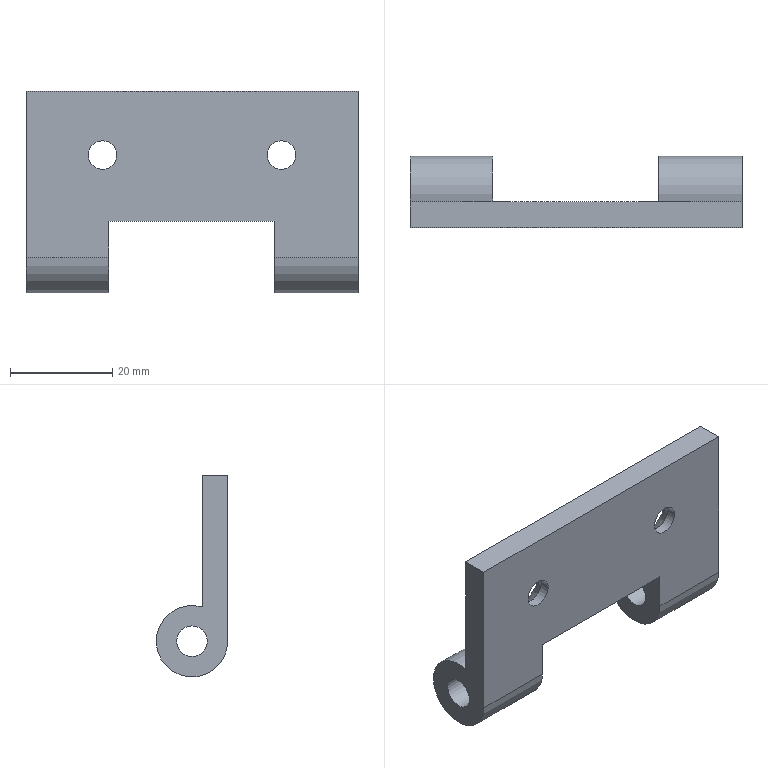Part | NX | 1 solid | 16 faces | box 65 x 14 x 39.5 mm | volume 12285 mm3 | plane 8 | cylinder 6 | cone 2 | commonest cylinder face diameters 5.6 x2 6 x2 14 x2
STEP:
#1=CARTESIAN_POINT('',(50.,0.,22.8));
#2=VERTEX_POINT('',#1);
#3=CARTESIAN_POINT('',(50.,0.,20.));
#4=DIRECTION('',(0.,1.,0.));
#5=DIRECTION('',(0.,0.,1.));
#6=AXIS2_PLACEMENT_3D('',#3,#4,#5);
#7=CIRCLE('',#6,2.8);
#8=EDGE_CURVE('',#2,#2,#7,.T.);
#9=ORIENTED_EDGE('',*,*,#8,.T.);
#10=EDGE_LOOP('',(#9));
#11=FACE_BOUND('',#10,.T.);
#12=CARTESIAN_POINT('',(16.25,0.,7.));
#13=VERTEX_POINT('',#12);
#14=CARTESIAN_POINT('',(48.75,0.,7.));
#15=VERTEX_POINT('',#14);
#16=CARTESIAN_POINT('',(65.,0.,7.));
#17=DIRECTION('',(1.,0.,0.));
#18=VECTOR('',#17,1000.);
#19=LINE('',#16,#18);
#20=EDGE_CURVE('',#13,#15,#19,.T.);
#21=ORIENTED_EDGE('',*,*,#20,.T.);
#22=CARTESIAN_POINT('',(48.75,0.,0.));
#23=VERTEX_POINT('',#22);
#24=CARTESIAN_POINT('',(48.75,0.,32.5));
#25=DIRECTION('',(0.,0.,-1.));
#26=VECTOR('',#25,1000.);
#27=LINE('',#24,#26);
#28=EDGE_CURVE('',#15,#23,#27,.T.);
#29=ORIENTED_EDGE('',*,*,#28,.T.);
#30=CARTESIAN_POINT('',(65.,0.,0.));
#31=VERTEX_POINT('',#30);
#32=CARTESIAN_POINT('',(65.,0.,0.));
#33=DIRECTION('',(-1.,0.,0.));
#34=VECTOR('',#33,1000.);
#35=LINE('',#32,#34);
#36=EDGE_CURVE('',#31,#23,#35,.T.);
#37=ORIENTED_EDGE('',*,*,#36,.F.);
#38=CARTESIAN_POINT('',(65.,0.,32.5));
#39=VERTEX_POINT('',#38);
#40=CARTESIAN_POINT('',(65.,0.,32.5));
#41=DIRECTION('',(0.,0.,-1.));
#42=VECTOR('',#41,1000.);
#43=LINE('',#40,#42);
#44=EDGE_CURVE('',#39,#31,#43,.T.);
#45=ORIENTED_EDGE('',*,*,#44,.F.);
#46=CARTESIAN_POINT('',(0.,0.,32.5));
#47=VERTEX_POINT('',#46);
#48=CARTESIAN_POINT('',(65.,0.,32.5));
#49=DIRECTION('',(-1.,0.,0.));
#50=VECTOR('',#49,1000.);
#51=LINE('',#48,#50);
#52=EDGE_CURVE('',#39,#47,#51,.T.);
#53=ORIENTED_EDGE('',*,*,#52,.T.);
#54=CARTESIAN_POINT('',(0.,0.,0.));
#55=VERTEX_POINT('',#54);
#56=CARTESIAN_POINT('',(0.,0.,32.5));
#57=DIRECTION('',(0.,0.,-1.));
#58=VECTOR('',#57,1000.);
#59=LINE('',#56,#58);
#60=EDGE_CURVE('',#47,#55,#59,.T.);
#61=ORIENTED_EDGE('',*,*,#60,.T.);
#62=CARTESIAN_POINT('',(16.25,0.,0.));
#63=VERTEX_POINT('',#62);
#64=CARTESIAN_POINT('',(65.,0.,0.));
#65=DIRECTION('',(-1.,0.,0.));
#66=VECTOR('',#65,1000.);
#67=LINE('',#64,#66);
#68=EDGE_CURVE('',#63,#55,#67,.T.);
#69=ORIENTED_EDGE('',*,*,#68,.F.);
#70=CARTESIAN_POINT('',(16.25,0.,32.5));
#71=DIRECTION('',(0.,0.,1.));
#72=VECTOR('',#71,1000.);
#73=LINE('',#70,#72);
#74=EDGE_CURVE('',#63,#13,#73,.T.);
#75=ORIENTED_EDGE('',*,*,#74,.T.);
#76=EDGE_LOOP('',(#21,#29,#37,#45,#53,#61,#69,#75));
#77=FACE_BOUND('',#76,.T.);
#78=CARTESIAN_POINT('',(15.,0.,22.8));
#79=VERTEX_POINT('',#78);
#80=CARTESIAN_POINT('',(15.,0.,20.));
#81=DIRECTION('',(0.,1.,0.));
#82=DIRECTION('',(0.,0.,1.));
#83=AXIS2_PLACEMENT_3D('',#80,#81,#82);
#84=CIRCLE('',#83,2.8);
#85=EDGE_CURVE('',#79,#79,#84,.T.);
#86=ORIENTED_EDGE('',*,*,#85,.T.);
#87=EDGE_LOOP('',(#86));
#88=FACE_BOUND('',#87,.T.);
#89=CARTESIAN_POINT('',(65.,0.,32.5));
#90=DIRECTION('',(0.,1.,0.));
#91=DIRECTION('',(0.,0.,1.));
#92=AXIS2_PLACEMENT_3D('',#89,#90,#91);
#93=PLANE('',#92);
#94=ADVANCED_FACE('',(#11,#77,#88),#93,.F.);
#95=CARTESIAN_POINT('',(50.,5.,25.3));
#96=VERTEX_POINT('',#95);
#97=CARTESIAN_POINT('',(50.,5.,20.));
#98=DIRECTION('',(0.,1.,0.));
#99=DIRECTION('',(0.,0.,1.));
#100=AXIS2_PLACEMENT_3D('',#97,#98,#99);
#101=CIRCLE('',#100,5.3);
#102=EDGE_CURVE('',#96,#96,#101,.T.);
#103=ORIENTED_EDGE('',*,*,#102,.F.);
#104=EDGE_LOOP('',(#103));
#105=FACE_BOUND('',#104,.T.);
#106=CARTESIAN_POINT('',(65.,5.,6.708));
#107=VERTEX_POINT('',#106);
#108=CARTESIAN_POINT('',(48.75,5.,6.708));
#109=VERTEX_POINT('',#108);
#110=CARTESIAN_POINT('',(65.,5.,6.708));
#111=DIRECTION('',(-1.,0.,0.));
#112=VECTOR('',#111,1000.);
#113=LINE('',#110,#112);
#114=EDGE_CURVE('',#107,#109,#113,.T.);
#115=ORIENTED_EDGE('',*,*,#114,.T.);
#116=CARTESIAN_POINT('',(48.75,5.,7.));
#117=VERTEX_POINT('',#116);
#118=CARTESIAN_POINT('',(48.75,5.,6.708));
#119=DIRECTION('',(0.,0.,1.));
#120=VECTOR('',#119,1000.);
#121=LINE('',#118,#120);
#122=EDGE_CURVE('',#109,#117,#121,.T.);
#123=ORIENTED_EDGE('',*,*,#122,.T.);
#124=CARTESIAN_POINT('',(16.25,5.,7.));
#125=VERTEX_POINT('',#124);
#126=CARTESIAN_POINT('',(65.,5.,7.));
#127=DIRECTION('',(-1.,0.,0.));
#128=VECTOR('',#127,1000.);
#129=LINE('',#126,#128);
#130=EDGE_CURVE('',#117,#125,#129,.T.);
#131=ORIENTED_EDGE('',*,*,#130,.T.);
#132=CARTESIAN_POINT('',(16.25,5.,6.708));
#133=VERTEX_POINT('',#132);
#134=CARTESIAN_POINT('',(16.25,5.,6.708));
#135=DIRECTION('',(0.,0.,-1.));
#136=VECTOR('',#135,1000.);
#137=LINE('',#134,#136);
#138=EDGE_CURVE('',#125,#133,#137,.T.);
#139=ORIENTED_EDGE('',*,*,#138,.T.);
#140=CARTESIAN_POINT('',(0.,5.,6.708));
#141=VERTEX_POINT('',#140);
#142=CARTESIAN_POINT('',(65.,5.,6.708));
#143=DIRECTION('',(-1.,0.,0.));
#144=VECTOR('',#143,1000.);
#145=LINE('',#142,#144);
#146=EDGE_CURVE('',#133,#141,#145,.T.);
#147=ORIENTED_EDGE('',*,*,#146,.T.);
#148=CARTESIAN_POINT('',(0.,5.,32.5));
#149=VERTEX_POINT('',#148);
#150=CARTESIAN_POINT('',(0.,5.,6.708));
#151=DIRECTION('',(0.,0.,1.));
#152=VECTOR('',#151,1000.);
#153=LINE('',#150,#152);
#154=EDGE_CURVE('',#141,#149,#153,.T.);
#155=ORIENTED_EDGE('',*,*,#154,.T.);
#156=CARTESIAN_POINT('',(65.,5.,32.5));
#157=VERTEX_POINT('',#156);
#158=CARTESIAN_POINT('',(65.,5.,32.5));
#159=DIRECTION('',(-1.,0.,0.));
#160=VECTOR('',#159,1000.);
#161=LINE('',#158,#160);
#162=EDGE_CURVE('',#157,#149,#161,.T.);
#163=ORIENTED_EDGE('',*,*,#162,.F.);
#164=CARTESIAN_POINT('',(65.,5.,6.708));
#165=DIRECTION('',(0.,0.,1.));
#166=VECTOR('',#165,1000.);
#167=LINE('',#164,#166);
#168=EDGE_CURVE('',#107,#157,#167,.T.);
#169=ORIENTED_EDGE('',*,*,#168,.F.);
#170=EDGE_LOOP('',(#115,#123,#131,#139,#147,#155,#163,#169));
#171=FACE_BOUND('',#170,.T.);
#172=CARTESIAN_POINT('',(15.,5.,25.3));
#173=VERTEX_POINT('',#172);
#174=CARTESIAN_POINT('',(15.,5.,20.));
#175=DIRECTION('',(0.,1.,0.));
#176=DIRECTION('',(0.,0.,1.));
#177=AXIS2_PLACEMENT_3D('',#174,#175,#176);
#178=CIRCLE('',#177,5.3);
#179=EDGE_CURVE('',#173,#173,#178,.T.);
#180=ORIENTED_EDGE('',*,*,#179,.F.);
#181=EDGE_LOOP('',(#180));
#182=FACE_BOUND('',#181,.T.);
#183=CARTESIAN_POINT('',(65.,5.,6.708));
#184=DIRECTION('',(0.,-1.,0.));
#185=DIRECTION('',(0.,0.,-1.));
#186=AXIS2_PLACEMENT_3D('',#183,#184,#185);
#187=PLANE('',#186);
#188=ADVANCED_FACE('',(#105,#171,#182),#187,.F.);
#189=ORIENTED_EDGE('',*,*,#114,.F.);
#190=CARTESIAN_POINT('',(65.,7.,0.));
#191=DIRECTION('',(1.,0.,0.));
#192=DIRECTION('',(0.,0.,-1.));
#193=AXIS2_PLACEMENT_3D('',#190,#191,#192);
#194=CIRCLE('',#193,7.);
#195=EDGE_CURVE('',#31,#107,#194,.T.);
#196=ORIENTED_EDGE('',*,*,#195,.F.);
#197=ORIENTED_EDGE('',*,*,#36,.T.);
#198=CARTESIAN_POINT('',(48.75,7.,0.));
#199=DIRECTION('',(1.,0.,0.));
#200=DIRECTION('',(0.,0.,-1.));
#201=AXIS2_PLACEMENT_3D('',#198,#199,#200);
#202=CIRCLE('',#201,7.);
#203=EDGE_CURVE('',#23,#109,#202,.T.);
#204=ORIENTED_EDGE('',*,*,#203,.T.);
#205=EDGE_LOOP('',(#189,#196,#197,#204));
#206=FACE_BOUND('',#205,.T.);
#207=CARTESIAN_POINT('',(65.,7.,0.));
#208=DIRECTION('',(-1.,0.,0.));
#209=DIRECTION('',(0.,0.,1.));
#210=AXIS2_PLACEMENT_3D('',#207,#208,#209);
#211=CYLINDRICAL_SURFACE('',#210,7.);
#212=ADVANCED_FACE('',(#206),#211,.T.);
#213=CARTESIAN_POINT('',(48.75,7.,-3.));
#214=VERTEX_POINT('',#213);
#215=CARTESIAN_POINT('',(48.75,7.,0.));
#216=DIRECTION('',(1.,0.,0.));
#217=DIRECTION('',(0.,0.,-1.));
#218=AXIS2_PLACEMENT_3D('',#215,#216,#217);
#219=CIRCLE('',#218,3.);
#220=EDGE_CURVE('',#214,#214,#219,.T.);
#221=ORIENTED_EDGE('',*,*,#220,.F.);
#222=EDGE_LOOP('',(#221));
#223=FACE_BOUND('',#222,.T.);
#224=CARTESIAN_POINT('',(65.,7.,-3.));
#225=VERTEX_POINT('',#224);
#226=CARTESIAN_POINT('',(65.,7.,0.));
#227=DIRECTION('',(1.,0.,0.));
#228=DIRECTION('',(0.,0.,-1.));
#229=AXIS2_PLACEMENT_3D('',#226,#227,#228);
#230=CIRCLE('',#229,3.);
#231=EDGE_CURVE('',#225,#225,#230,.T.);
#232=ORIENTED_EDGE('',*,*,#231,.T.);
#233=EDGE_LOOP('',(#232));
#234=FACE_BOUND('',#233,.T.);
#235=CARTESIAN_POINT('',(65.,7.,0.));
#236=DIRECTION('',(-1.,0.,0.));
#237=DIRECTION('',(0.,0.,1.));
#238=AXIS2_PLACEMENT_3D('',#235,#236,#237);
#239=CYLINDRICAL_SURFACE('',#238,3.);
#240=ADVANCED_FACE('',(#223,#234),#239,.F.);
#241=CARTESIAN_POINT('',(65.,5.,32.5));
#242=DIRECTION('',(0.,-1.,0.));
#243=VECTOR('',#242,1000.);
#244=LINE('',#241,#243);
#245=EDGE_CURVE('',#157,#39,#244,.T.);
#246=ORIENTED_EDGE('',*,*,#245,.T.);
#247=ORIENTED_EDGE('',*,*,#44,.T.);
#248=ORIENTED_EDGE('',*,*,#195,.T.);
#249=ORIENTED_EDGE('',*,*,#168,.T.);
#250=EDGE_LOOP('',(#246,#247,#248,#249));
#251=FACE_BOUND('',#250,.T.);
#252=ORIENTED_EDGE('',*,*,#231,.F.);
#253=EDGE_LOOP('',(#252));
#254=FACE_BOUND('',#253,.T.);
#255=CARTESIAN_POINT('',(65.,7.,0.));
#256=DIRECTION('',(1.,0.,0.));
#257=DIRECTION('',(0.,0.,-1.));
#258=AXIS2_PLACEMENT_3D('',#255,#256,#257);
#259=PLANE('',#258);
#260=ADVANCED_FACE('',(#251,#254),#259,.T.);
#261=CARTESIAN_POINT('',(0.,5.,32.5));
#262=DIRECTION('',(0.,-1.,0.));
#263=VECTOR('',#262,1000.);
#264=LINE('',#261,#263);
#265=EDGE_CURVE('',#149,#47,#264,.T.);
#266=ORIENTED_EDGE('',*,*,#265,.F.);
#267=ORIENTED_EDGE('',*,*,#154,.F.);
#268=CARTESIAN_POINT('',(0.,7.,0.));
#269=DIRECTION('',(1.,0.,0.));
#270=DIRECTION('',(0.,0.,-1.));
#271=AXIS2_PLACEMENT_3D('',#268,#269,#270);
#272=CIRCLE('',#271,7.);
#273=EDGE_CURVE('',#55,#141,#272,.T.);
#274=ORIENTED_EDGE('',*,*,#273,.F.);
#275=ORIENTED_EDGE('',*,*,#60,.F.);
#276=EDGE_LOOP('',(#266,#267,#274,#275));
#277=FACE_BOUND('',#276,.T.);
#278=CARTESIAN_POINT('',(0.,7.,-3.));
#279=VERTEX_POINT('',#278);
#280=CARTESIAN_POINT('',(0.,7.,0.));
#281=DIRECTION('',(1.,0.,0.));
#282=DIRECTION('',(0.,0.,-1.));
#283=AXIS2_PLACEMENT_3D('',#280,#281,#282);
#284=CIRCLE('',#283,3.);
#285=EDGE_CURVE('',#279,#279,#284,.T.);
#286=ORIENTED_EDGE('',*,*,#285,.T.);
#287=EDGE_LOOP('',(#286));
#288=FACE_BOUND('',#287,.T.);
#289=CARTESIAN_POINT('',(0.,7.,0.));
#290=DIRECTION('',(1.,0.,0.));
#291=DIRECTION('',(0.,0.,-1.));
#292=AXIS2_PLACEMENT_3D('',#289,#290,#291);
#293=PLANE('',#292);
#294=ADVANCED_FACE('',(#277,#288),#293,.F.);
#295=ORIENTED_EDGE('',*,*,#265,.T.);
#296=ORIENTED_EDGE('',*,*,#52,.F.);
#297=ORIENTED_EDGE('',*,*,#245,.F.);
#298=ORIENTED_EDGE('',*,*,#162,.T.);
#299=EDGE_LOOP('',(#295,#296,#297,#298));
#300=FACE_BOUND('',#299,.T.);
#301=CARTESIAN_POINT('',(65.,5.,32.5));
#302=DIRECTION('',(0.,0.,-1.));
#303=DIRECTION('',(-1.,0.,0.));
#304=AXIS2_PLACEMENT_3D('',#301,#302,#303);
#305=PLANE('',#304);
#306=ADVANCED_FACE('',(#300),#305,.F.);
#307=ORIENTED_EDGE('',*,*,#273,.T.);
#308=ORIENTED_EDGE('',*,*,#146,.F.);
#309=CARTESIAN_POINT('',(16.25,7.,0.));
#310=DIRECTION('',(-1.,0.,0.));
#311=DIRECTION('',(0.,0.,1.));
#312=AXIS2_PLACEMENT_3D('',#309,#310,#311);
#313=CIRCLE('',#312,7.);
#314=EDGE_CURVE('',#133,#63,#313,.T.);
#315=ORIENTED_EDGE('',*,*,#314,.T.);
#316=ORIENTED_EDGE('',*,*,#68,.T.);
#317=EDGE_LOOP('',(#307,#308,#315,#316));
#318=FACE_BOUND('',#317,.T.);
#319=CARTESIAN_POINT('',(65.,7.,0.));
#320=DIRECTION('',(-1.,0.,0.));
#321=DIRECTION('',(0.,0.,1.));
#322=AXIS2_PLACEMENT_3D('',#319,#320,#321);
#323=CYLINDRICAL_SURFACE('',#322,7.);
#324=ADVANCED_FACE('',(#318),#323,.T.);
#325=CARTESIAN_POINT('',(16.25,7.,3.));
#326=VERTEX_POINT('',#325);
#327=CARTESIAN_POINT('',(16.25,7.,0.));
#328=DIRECTION('',(-1.,0.,0.));
#329=DIRECTION('',(0.,0.,1.));
#330=AXIS2_PLACEMENT_3D('',#327,#328,#329);
#331=CIRCLE('',#330,3.);
#332=EDGE_CURVE('',#326,#326,#331,.T.);
#333=ORIENTED_EDGE('',*,*,#332,.F.);
#334=EDGE_LOOP('',(#333));
#335=FACE_BOUND('',#334,.T.);
#336=ORIENTED_EDGE('',*,*,#285,.F.);
#337=EDGE_LOOP('',(#336));
#338=FACE_BOUND('',#337,.T.);
#339=CARTESIAN_POINT('',(65.,7.,0.));
#340=DIRECTION('',(-1.,0.,0.));
#341=DIRECTION('',(0.,0.,1.));
#342=AXIS2_PLACEMENT_3D('',#339,#340,#341);
#343=CYLINDRICAL_SURFACE('',#342,3.);
#344=ADVANCED_FACE('',(#335,#338),#343,.F.);
#345=CARTESIAN_POINT('',(16.25,-65.,7.));
#346=DIRECTION('',(0.,1.,0.));
#347=VECTOR('',#346,1000.);
#348=LINE('',#345,#347);
#349=EDGE_CURVE('',#13,#125,#348,.T.);
#350=ORIENTED_EDGE('',*,*,#349,.T.);
#351=ORIENTED_EDGE('',*,*,#130,.F.);
#352=CARTESIAN_POINT('',(48.75,-65.,7.));
#353=DIRECTION('',(0.,1.,0.));
#354=VECTOR('',#353,1000.);
#355=LINE('',#352,#354);
#356=EDGE_CURVE('',#15,#117,#355,.T.);
#357=ORIENTED_EDGE('',*,*,#356,.F.);
#358=ORIENTED_EDGE('',*,*,#20,.F.);
#359=EDGE_LOOP('',(#350,#351,#357,#358));
#360=FACE_BOUND('',#359,.T.);
#361=CARTESIAN_POINT('',(16.25,-65.,7.));
#362=DIRECTION('',(0.,0.,1.));
#363=DIRECTION('',(1.,0.,0.));
#364=AXIS2_PLACEMENT_3D('',#361,#362,#363);
#365=PLANE('',#364);
#366=ADVANCED_FACE('',(#360),#365,.F.);
#367=ORIENTED_EDGE('',*,*,#220,.T.);
#368=EDGE_LOOP('',(#367));
#369=FACE_BOUND('',#368,.T.);
#370=ORIENTED_EDGE('',*,*,#356,.T.);
#371=ORIENTED_EDGE('',*,*,#122,.F.);
#372=ORIENTED_EDGE('',*,*,#203,.F.);
#373=ORIENTED_EDGE('',*,*,#28,.F.);
#374=EDGE_LOOP('',(#370,#371,#372,#373));
#375=FACE_BOUND('',#374,.T.);
#376=CARTESIAN_POINT('',(48.75,-65.,7.));
#377=DIRECTION('',(1.,0.,0.));
#378=DIRECTION('',(0.,0.,-1.));
#379=AXIS2_PLACEMENT_3D('',#376,#377,#378);
#380=PLANE('',#379);
#381=ADVANCED_FACE('',(#369,#375),#380,.F.);
#382=ORIENTED_EDGE('',*,*,#332,.T.);
#383=EDGE_LOOP('',(#382));
#384=FACE_BOUND('',#383,.T.);
#385=ORIENTED_EDGE('',*,*,#314,.F.);
#386=ORIENTED_EDGE('',*,*,#138,.F.);
#387=ORIENTED_EDGE('',*,*,#349,.F.);
#388=ORIENTED_EDGE('',*,*,#74,.F.);
#389=EDGE_LOOP('',(#385,#386,#387,#388));
#390=FACE_BOUND('',#389,.T.);
#391=CARTESIAN_POINT('',(16.25,-65.,-7.));
#392=DIRECTION('',(-1.,0.,0.));
#393=DIRECTION('',(0.,0.,1.));
#394=AXIS2_PLACEMENT_3D('',#391,#392,#393);
#395=PLANE('',#394);
#396=ADVANCED_FACE('',(#384,#390),#395,.F.);
#397=ORIENTED_EDGE('',*,*,#102,.T.);
#398=EDGE_LOOP('',(#397));
#399=FACE_BOUND('',#398,.T.);
#400=CARTESIAN_POINT('',(50.,1.913,22.8));
#401=VERTEX_POINT('',#400);
#402=CARTESIAN_POINT('',(50.,1.913,20.));
#403=DIRECTION('',(0.,1.,0.));
#404=DIRECTION('',(0.,0.,1.));
#405=AXIS2_PLACEMENT_3D('',#402,#403,#404);
#406=CIRCLE('',#405,2.8);
#407=EDGE_CURVE('',#401,#401,#406,.T.);
#408=ORIENTED_EDGE('',*,*,#407,.F.);
#409=EDGE_LOOP('',(#408));
#410=FACE_BOUND('',#409,.T.);
#411=CARTESIAN_POINT('',(50.,1.913,20.));
#412=DIRECTION('',(0.,1.,0.));
#413=DIRECTION('',(0.,0.,1.));
#414=AXIS2_PLACEMENT_3D('',#411,#412,#413);
#415=CONICAL_SURFACE('',#414,2.8,0.6807);
#416=ADVANCED_FACE('',(#399,#410),#415,.F.);
#417=ORIENTED_EDGE('',*,*,#407,.T.);
#418=EDGE_LOOP('',(#417));
#419=FACE_BOUND('',#418,.T.);
#420=ORIENTED_EDGE('',*,*,#8,.F.);
#421=EDGE_LOOP('',(#420));
#422=FACE_BOUND('',#421,.T.);
#423=CARTESIAN_POINT('',(50.,0.,20.));
#424=DIRECTION('',(0.,1.,0.));
#425=DIRECTION('',(0.,0.,1.));
#426=AXIS2_PLACEMENT_3D('',#423,#424,#425);
#427=CYLINDRICAL_SURFACE('',#426,2.8);
#428=ADVANCED_FACE('',(#419,#422),#427,.F.);
#429=ORIENTED_EDGE('',*,*,#179,.T.);
#430=EDGE_LOOP('',(#429));
#431=FACE_BOUND('',#430,.T.);
#432=CARTESIAN_POINT('',(15.,1.913,22.8));
#433=VERTEX_POINT('',#432);
#434=CARTESIAN_POINT('',(15.,1.913,20.));
#435=DIRECTION('',(0.,1.,0.));
#436=DIRECTION('',(0.,0.,1.));
#437=AXIS2_PLACEMENT_3D('',#434,#435,#436);
#438=CIRCLE('',#437,2.8);
#439=EDGE_CURVE('',#433,#433,#438,.T.);
#440=ORIENTED_EDGE('',*,*,#439,.F.);
#441=EDGE_LOOP('',(#440));
#442=FACE_BOUND('',#441,.T.);
#443=CARTESIAN_POINT('',(15.,1.913,20.));
#444=DIRECTION('',(0.,1.,0.));
#445=DIRECTION('',(0.,0.,1.));
#446=AXIS2_PLACEMENT_3D('',#443,#444,#445);
#447=CONICAL_SURFACE('',#446,2.8,0.6807);
#448=ADVANCED_FACE('',(#431,#442),#447,.F.);
#449=ORIENTED_EDGE('',*,*,#439,.T.);
#450=EDGE_LOOP('',(#449));
#451=FACE_BOUND('',#450,.T.);
#452=ORIENTED_EDGE('',*,*,#85,.F.);
#453=EDGE_LOOP('',(#452));
#454=FACE_BOUND('',#453,.T.);
#455=CARTESIAN_POINT('',(15.,0.,20.));
#456=DIRECTION('',(0.,1.,0.));
#457=DIRECTION('',(0.,0.,1.));
#458=AXIS2_PLACEMENT_3D('',#455,#456,#457);
#459=CYLINDRICAL_SURFACE('',#458,2.8);
#460=ADVANCED_FACE('',(#451,#454),#459,.F.);
#461=CLOSED_SHELL('',(#94,#188,#212,#240,#260,#294,#306,#324,#344,#366,#381,#396,#416,#428,#448,#460));
#462=MANIFOLD_SOLID_BREP('',#461);
#463=(LENGTH_UNIT()NAMED_UNIT(*)SI_UNIT(.MILLI.,.METRE.));
#464=UNCERTAINTY_MEASURE_WITH_UNIT(LENGTH_MEASURE(0.00001),#463,'','');
#465=(NAMED_UNIT(*)PLANE_ANGLE_UNIT()SI_UNIT($,.RADIAN.));
#466=(NAMED_UNIT(*)SI_UNIT($,.STERADIAN.)SOLID_ANGLE_UNIT());
#467=(GEOMETRIC_REPRESENTATION_CONTEXT(3)GLOBAL_UNCERTAINTY_ASSIGNED_CONTEXT((#464))GLOBAL_UNIT_ASSIGNED_CONTEXT((#463,#465,#466))REPRESENTATION_CONTEXT('',''));
#468=ADVANCED_BREP_SHAPE_REPRESENTATION('',(#462),#467);